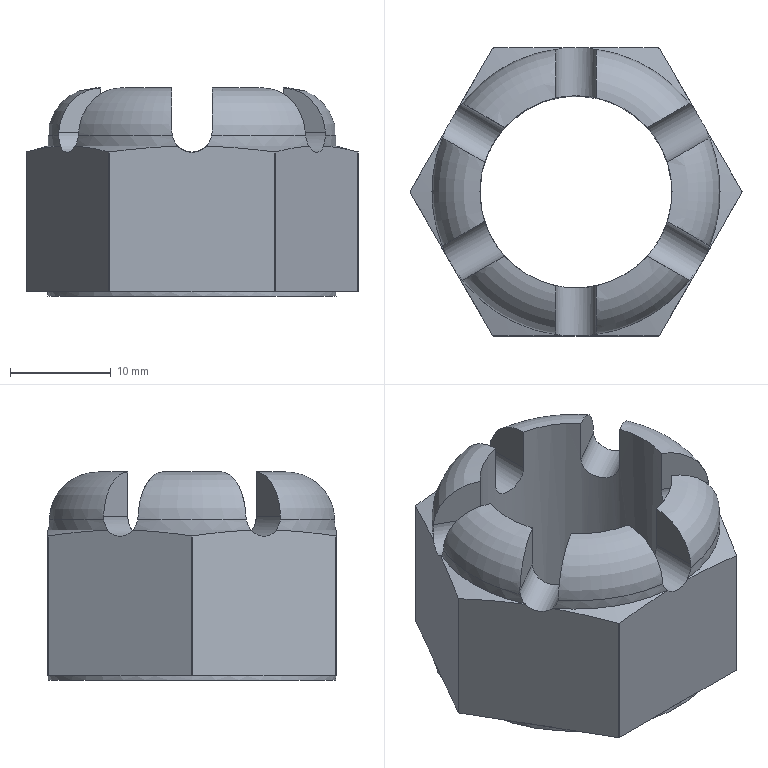Part | NX | features solid 2 | 1 solid | 57 faces | box 32.941 x 28.575 x 20.638 mm | volume 7329 mm3 | plane 25 | cylinder 20 | torus 6 | cone 6 | commonest cylinder face diameters 28.575 x7 3.969 x6 32.941 x6 19.05 x1